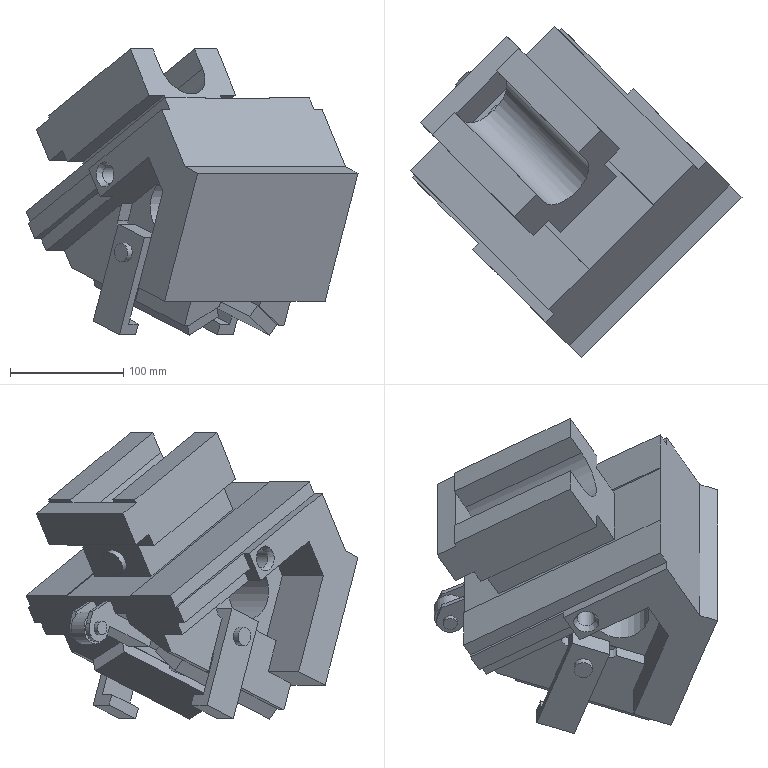Part | NX | features solid 2 | 1 solid | 154 faces | box 292.654 x 292.654 x 252.319 mm | volume 4236624 mm3 | plane 132 | cylinder 18 | cone 4 | commonest cylinder face diameters 16 x5 20 x4 12 x2 24 x2 22 x1 28 x1